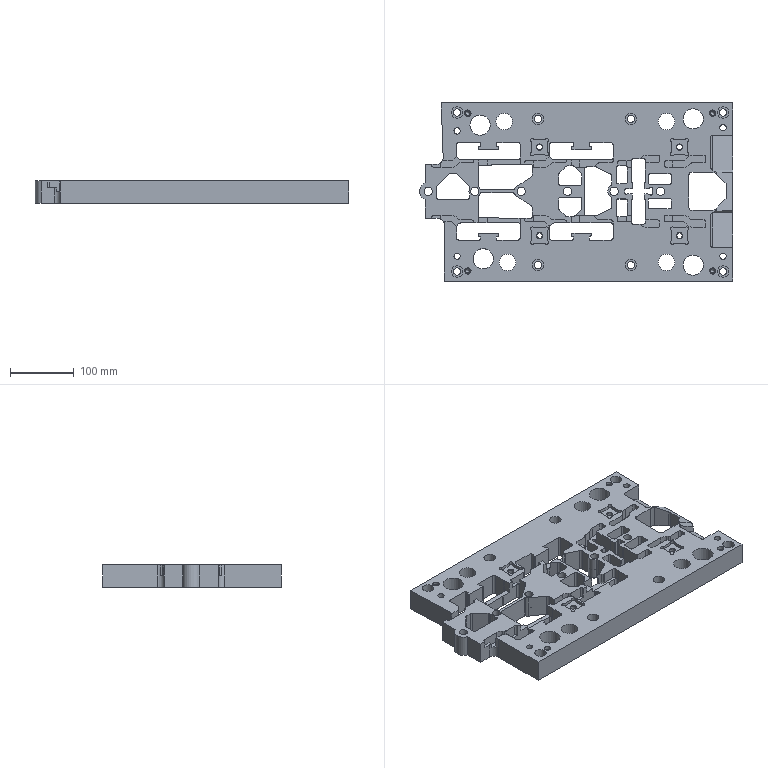Part | NX | features DIE-80 2 | 1 solid | 612 faces | box 492.396 x 280 x 35 mm | volume 3008147 mm3 | plane 311 | cylinder 281 | spline 12 | cone 8 | commonest cylinder face diameters 6 x99 10 x26 18 x19 1.76 x16 2 x16 26 x15